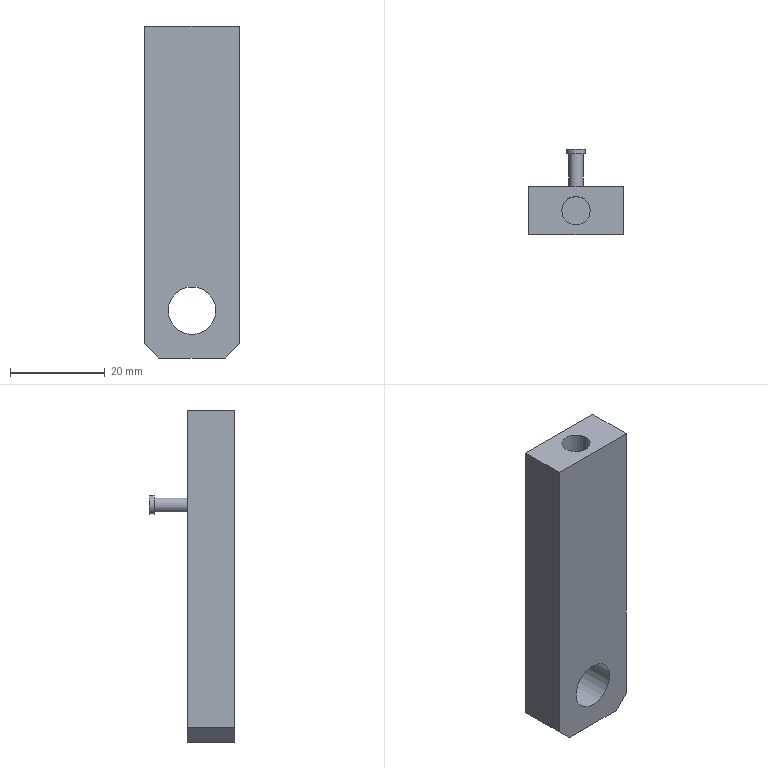Part | NX | features DATUM_CSYS 4, EXTRUDE 3, SKETCH 3, HOLE PACKAGE 1, SIMPLE HOLE 1 | 1 solid | 15 faces | box 20 x 18 x 70 mm | volume 11773 mm3 | plane 11 | cylinder 4 | commonest cylinder face diameters 3 x1 4 x1 6 x1 10 x1
STEP:
#1=CARTESIAN_POINT('',(-10.,5.,0.));
#2=VERTEX_POINT('',#1);
#3=CARTESIAN_POINT('',(-10.,5.,-67.));
#4=VERTEX_POINT('',#3);
#5=CARTESIAN_POINT('',(-10.,5.,0.));
#6=DIRECTION('',(0.,0.,-1.));
#7=VECTOR('',#6,1000.);
#8=LINE('',#5,#7);
#9=EDGE_CURVE('',#2,#4,#8,.T.);
#10=ORIENTED_EDGE('',*,*,#9,.T.);
#11=CARTESIAN_POINT('',(-10.,-5.,-67.));
#12=VERTEX_POINT('',#11);
#13=CARTESIAN_POINT('',(-10.,-5.,-67.));
#14=DIRECTION('',(0.,1.,0.));
#15=VECTOR('',#14,1000.);
#16=LINE('',#13,#15);
#17=EDGE_CURVE('',#12,#4,#16,.T.);
#18=ORIENTED_EDGE('',*,*,#17,.F.);
#19=CARTESIAN_POINT('',(-10.,-5.,0.));
#20=VERTEX_POINT('',#19);
#21=CARTESIAN_POINT('',(-10.,-5.,0.));
#22=DIRECTION('',(0.,0.,-1.));
#23=VECTOR('',#22,1000.);
#24=LINE('',#21,#23);
#25=EDGE_CURVE('',#20,#12,#24,.T.);
#26=ORIENTED_EDGE('',*,*,#25,.F.);
#27=CARTESIAN_POINT('',(-10.,-5.,0.));
#28=DIRECTION('',(0.,1.,0.));
#29=VECTOR('',#28,1000.);
#30=LINE('',#27,#29);
#31=EDGE_CURVE('',#20,#2,#30,.T.);
#32=ORIENTED_EDGE('',*,*,#31,.T.);
#33=EDGE_LOOP('',(#10,#18,#26,#32));
#34=FACE_BOUND('',#33,.T.);
#35=CARTESIAN_POINT('',(-10.,-5.,0.));
#36=DIRECTION('',(1.,0.,0.));
#37=DIRECTION('',(0.,0.,-1.));
#38=AXIS2_PLACEMENT_3D('',#35,#36,#37);
#39=PLANE('',#38);
#40=ADVANCED_FACE('',(#34),#39,.F.);
#41=CARTESIAN_POINT('',(-7.,5.,-70.));
#42=VERTEX_POINT('',#41);
#43=CARTESIAN_POINT('',(-10.,5.,-67.));
#44=DIRECTION('',(0.7071,0.,-0.7071));
#45=VECTOR('',#44,1000.);
#46=LINE('',#43,#45);
#47=EDGE_CURVE('',#4,#42,#46,.T.);
#48=ORIENTED_EDGE('',*,*,#47,.T.);
#49=CARTESIAN_POINT('',(-7.,-5.,-70.));
#50=VERTEX_POINT('',#49);
#51=CARTESIAN_POINT('',(-7.,-5.,-70.));
#52=DIRECTION('',(0.,1.,0.));
#53=VECTOR('',#52,1000.);
#54=LINE('',#51,#53);
#55=EDGE_CURVE('',#50,#42,#54,.T.);
#56=ORIENTED_EDGE('',*,*,#55,.F.);
#57=CARTESIAN_POINT('',(-10.,-5.,-67.));
#58=DIRECTION('',(0.7071,0.,-0.7071));
#59=VECTOR('',#58,1000.);
#60=LINE('',#57,#59);
#61=EDGE_CURVE('',#12,#50,#60,.T.);
#62=ORIENTED_EDGE('',*,*,#61,.F.);
#63=ORIENTED_EDGE('',*,*,#17,.T.);
#64=EDGE_LOOP('',(#48,#56,#62,#63));
#65=FACE_BOUND('',#64,.T.);
#66=CARTESIAN_POINT('',(-10.,-5.,-67.));
#67=DIRECTION('',(0.7071,0.,0.7071));
#68=DIRECTION('',(0.7071,0.,-0.7071));
#69=AXIS2_PLACEMENT_3D('',#66,#67,#68);
#70=PLANE('',#69);
#71=ADVANCED_FACE('',(#65),#70,.F.);
#72=CARTESIAN_POINT('',(7.,5.,-70.));
#73=VERTEX_POINT('',#72);
#74=CARTESIAN_POINT('',(-7.,5.,-70.));
#75=DIRECTION('',(1.,0.,0.));
#76=VECTOR('',#75,1000.);
#77=LINE('',#74,#76);
#78=EDGE_CURVE('',#42,#73,#77,.T.);
#79=ORIENTED_EDGE('',*,*,#78,.T.);
#80=CARTESIAN_POINT('',(7.,-5.,-70.));
#81=VERTEX_POINT('',#80);
#82=CARTESIAN_POINT('',(7.,-5.,-70.));
#83=DIRECTION('',(0.,1.,0.));
#84=VECTOR('',#83,1000.);
#85=LINE('',#82,#84);
#86=EDGE_CURVE('',#81,#73,#85,.T.);
#87=ORIENTED_EDGE('',*,*,#86,.F.);
#88=CARTESIAN_POINT('',(-7.,-5.,-70.));
#89=DIRECTION('',(1.,0.,0.));
#90=VECTOR('',#89,1000.);
#91=LINE('',#88,#90);
#92=EDGE_CURVE('',#50,#81,#91,.T.);
#93=ORIENTED_EDGE('',*,*,#92,.F.);
#94=ORIENTED_EDGE('',*,*,#55,.T.);
#95=EDGE_LOOP('',(#79,#87,#93,#94));
#96=FACE_BOUND('',#95,.T.);
#97=CARTESIAN_POINT('',(-7.,-5.,-70.));
#98=DIRECTION('',(0.,0.,1.));
#99=DIRECTION('',(1.,0.,0.));
#100=AXIS2_PLACEMENT_3D('',#97,#98,#99);
#101=PLANE('',#100);
#102=ADVANCED_FACE('',(#96),#101,.F.);
#103=CARTESIAN_POINT('',(10.,5.,-67.));
#104=VERTEX_POINT('',#103);
#105=CARTESIAN_POINT('',(7.,5.,-70.));
#106=DIRECTION('',(0.7071,0.,0.7071));
#107=VECTOR('',#106,1000.);
#108=LINE('',#105,#107);
#109=EDGE_CURVE('',#73,#104,#108,.T.);
#110=ORIENTED_EDGE('',*,*,#109,.T.);
#111=CARTESIAN_POINT('',(10.,-5.,-67.));
#112=VERTEX_POINT('',#111);
#113=CARTESIAN_POINT('',(10.,-5.,-67.));
#114=DIRECTION('',(0.,1.,0.));
#115=VECTOR('',#114,1000.);
#116=LINE('',#113,#115);
#117=EDGE_CURVE('',#112,#104,#116,.T.);
#118=ORIENTED_EDGE('',*,*,#117,.F.);
#119=CARTESIAN_POINT('',(7.,-5.,-70.));
#120=DIRECTION('',(0.7071,0.,0.7071));
#121=VECTOR('',#120,1000.);
#122=LINE('',#119,#121);
#123=EDGE_CURVE('',#81,#112,#122,.T.);
#124=ORIENTED_EDGE('',*,*,#123,.F.);
#125=ORIENTED_EDGE('',*,*,#86,.T.);
#126=EDGE_LOOP('',(#110,#118,#124,#125));
#127=FACE_BOUND('',#126,.T.);
#128=CARTESIAN_POINT('',(7.,-5.,-70.));
#129=DIRECTION('',(-0.7071,0.,0.7071));
#130=DIRECTION('',(0.7071,0.,0.7071));
#131=AXIS2_PLACEMENT_3D('',#128,#129,#130);
#132=PLANE('',#131);
#133=ADVANCED_FACE('',(#127),#132,.F.);
#134=CARTESIAN_POINT('',(10.,5.,0.));
#135=VERTEX_POINT('',#134);
#136=CARTESIAN_POINT('',(10.,5.,-67.));
#137=DIRECTION('',(0.,0.,1.));
#138=VECTOR('',#137,1000.);
#139=LINE('',#136,#138);
#140=EDGE_CURVE('',#104,#135,#139,.T.);
#141=ORIENTED_EDGE('',*,*,#140,.T.);
#142=CARTESIAN_POINT('',(10.,-5.,0.));
#143=VERTEX_POINT('',#142);
#144=CARTESIAN_POINT('',(10.,-5.,0.));
#145=DIRECTION('',(0.,1.,0.));
#146=VECTOR('',#145,1000.);
#147=LINE('',#144,#146);
#148=EDGE_CURVE('',#143,#135,#147,.T.);
#149=ORIENTED_EDGE('',*,*,#148,.F.);
#150=CARTESIAN_POINT('',(10.,-5.,-67.));
#151=DIRECTION('',(0.,0.,1.));
#152=VECTOR('',#151,1000.);
#153=LINE('',#150,#152);
#154=EDGE_CURVE('',#112,#143,#153,.T.);
#155=ORIENTED_EDGE('',*,*,#154,.F.);
#156=ORIENTED_EDGE('',*,*,#117,.T.);
#157=EDGE_LOOP('',(#141,#149,#155,#156));
#158=FACE_BOUND('',#157,.T.);
#159=CARTESIAN_POINT('',(10.,-5.,-67.));
#160=DIRECTION('',(-1.,0.,0.));
#161=DIRECTION('',(0.,0.,1.));
#162=AXIS2_PLACEMENT_3D('',#159,#160,#161);
#163=PLANE('',#162);
#164=ADVANCED_FACE('',(#158),#163,.F.);
#165=CARTESIAN_POINT('',(-3.,0.,0.));
#166=VERTEX_POINT('',#165);
#167=CARTESIAN_POINT('',(0.,0.,0.));
#168=DIRECTION('',(0.,0.,-1.));
#169=DIRECTION('',(-1.,0.,0.));
#170=AXIS2_PLACEMENT_3D('',#167,#168,#169);
#171=CIRCLE('',#170,3.);
#172=EDGE_CURVE('',#166,#166,#171,.T.);
#173=ORIENTED_EDGE('',*,*,#172,.T.);
#174=EDGE_LOOP('',(#173));
#175=FACE_BOUND('',#174,.T.);
#176=CARTESIAN_POINT('',(10.,5.,0.));
#177=DIRECTION('',(-1.,0.,0.));
#178=VECTOR('',#177,1000.);
#179=LINE('',#176,#178);
#180=EDGE_CURVE('',#135,#2,#179,.T.);
#181=ORIENTED_EDGE('',*,*,#180,.T.);
#182=ORIENTED_EDGE('',*,*,#31,.F.);
#183=CARTESIAN_POINT('',(10.,-5.,0.));
#184=DIRECTION('',(-1.,0.,0.));
#185=VECTOR('',#184,1000.);
#186=LINE('',#183,#185);
#187=EDGE_CURVE('',#143,#20,#186,.T.);
#188=ORIENTED_EDGE('',*,*,#187,.F.);
#189=ORIENTED_EDGE('',*,*,#148,.T.);
#190=EDGE_LOOP('',(#181,#182,#188,#189));
#191=FACE_BOUND('',#190,.T.);
#192=CARTESIAN_POINT('',(10.,-5.,0.));
#193=DIRECTION('',(0.,0.,-1.));
#194=DIRECTION('',(-1.,0.,0.));
#195=AXIS2_PLACEMENT_3D('',#192,#193,#194);
#196=PLANE('',#195);
#197=ADVANCED_FACE('',(#175,#191),#196,.F.);
#198=CARTESIAN_POINT('',(5.,-5.,-60.));
#199=VERTEX_POINT('',#198);
#200=CARTESIAN_POINT('',(0.,-5.,-60.));
#201=DIRECTION('',(0.,-1.,0.));
#202=DIRECTION('',(1.,0.,0.));
#203=AXIS2_PLACEMENT_3D('',#200,#201,#202);
#204=CIRCLE('',#203,5.);
#205=EDGE_CURVE('',#199,#199,#204,.T.);
#206=ORIENTED_EDGE('',*,*,#205,.T.);
#207=EDGE_LOOP('',(#206));
#208=FACE_BOUND('',#207,.T.);
#209=CARTESIAN_POINT('',(5.,5.,-60.));
#210=VERTEX_POINT('',#209);
#211=CARTESIAN_POINT('',(0.,5.,-60.));
#212=DIRECTION('',(0.,-1.,0.));
#213=DIRECTION('',(1.,0.,0.));
#214=AXIS2_PLACEMENT_3D('',#211,#212,#213);
#215=CIRCLE('',#214,5.);
#216=EDGE_CURVE('',#210,#210,#215,.T.);
#217=ORIENTED_EDGE('',*,*,#216,.F.);
#218=EDGE_LOOP('',(#217));
#219=FACE_BOUND('',#218,.T.);
#220=CARTESIAN_POINT('',(0.,-5.,-60.));
#221=DIRECTION('',(0.,1.,0.));
#222=DIRECTION('',(0.,0.,1.));
#223=AXIS2_PLACEMENT_3D('',#220,#221,#222);
#224=CYLINDRICAL_SURFACE('',#223,5.);
#225=ADVANCED_FACE('',(#208,#219),#224,.F.);
#226=ORIENTED_EDGE('',*,*,#25,.T.);
#227=ORIENTED_EDGE('',*,*,#61,.T.);
#228=ORIENTED_EDGE('',*,*,#92,.T.);
#229=ORIENTED_EDGE('',*,*,#123,.T.);
#230=ORIENTED_EDGE('',*,*,#154,.T.);
#231=ORIENTED_EDGE('',*,*,#187,.T.);
#232=EDGE_LOOP('',(#226,#227,#228,#229,#230,#231));
#233=FACE_BOUND('',#232,.T.);
#234=ORIENTED_EDGE('',*,*,#205,.F.);
#235=EDGE_LOOP('',(#234));
#236=FACE_BOUND('',#235,.T.);
#237=CARTESIAN_POINT('',(0.,-5.,-60.));
#238=DIRECTION('',(0.,-1.,0.));
#239=DIRECTION('',(0.,0.,-1.));
#240=AXIS2_PLACEMENT_3D('',#237,#238,#239);
#241=PLANE('',#240);
#242=ADVANCED_FACE('',(#233,#236),#241,.T.);
#243=CARTESIAN_POINT('',(1.5,5.,-20.));
#244=VERTEX_POINT('',#243);
#245=CARTESIAN_POINT('',(0.,5.,-20.));
#246=DIRECTION('',(0.,-1.,0.));
#247=DIRECTION('',(1.,0.,0.));
#248=AXIS2_PLACEMENT_3D('',#245,#246,#247);
#249=CIRCLE('',#248,1.5);
#250=EDGE_CURVE('',#244,#244,#249,.T.);
#251=ORIENTED_EDGE('',*,*,#250,.T.);
#252=EDGE_LOOP('',(#251));
#253=FACE_BOUND('',#252,.T.);
#254=ORIENTED_EDGE('',*,*,#9,.F.);
#255=ORIENTED_EDGE('',*,*,#180,.F.);
#256=ORIENTED_EDGE('',*,*,#140,.F.);
#257=ORIENTED_EDGE('',*,*,#109,.F.);
#258=ORIENTED_EDGE('',*,*,#78,.F.);
#259=ORIENTED_EDGE('',*,*,#47,.F.);
#260=EDGE_LOOP('',(#254,#255,#256,#257,#258,#259));
#261=FACE_BOUND('',#260,.T.);
#262=ORIENTED_EDGE('',*,*,#216,.T.);
#263=EDGE_LOOP('',(#262));
#264=FACE_BOUND('',#263,.T.);
#265=CARTESIAN_POINT('',(0.,5.,-60.));
#266=DIRECTION('',(0.,-1.,0.));
#267=DIRECTION('',(0.,0.,-1.));
#268=AXIS2_PLACEMENT_3D('',#265,#266,#267);
#269=PLANE('',#268);
#270=ADVANCED_FACE('',(#253,#261,#264),#269,.F.);
#271=CARTESIAN_POINT('',(1.5,12.,-20.));
#272=VERTEX_POINT('',#271);
#273=CARTESIAN_POINT('',(0.,12.,-20.));
#274=DIRECTION('',(0.,-1.,0.));
#275=DIRECTION('',(1.,0.,0.));
#276=AXIS2_PLACEMENT_3D('',#273,#274,#275);
#277=CIRCLE('',#276,1.5);
#278=EDGE_CURVE('',#272,#272,#277,.T.);
#279=ORIENTED_EDGE('',*,*,#278,.T.);
#280=EDGE_LOOP('',(#279));
#281=FACE_BOUND('',#280,.T.);
#282=ORIENTED_EDGE('',*,*,#250,.F.);
#283=EDGE_LOOP('',(#282));
#284=FACE_BOUND('',#283,.T.);
#285=CARTESIAN_POINT('',(0.,12.,-20.));
#286=DIRECTION('',(0.,-1.,0.));
#287=DIRECTION('',(0.,0.,-1.));
#288=AXIS2_PLACEMENT_3D('',#285,#286,#287);
#289=CYLINDRICAL_SURFACE('',#288,1.5);
#290=ADVANCED_FACE('',(#281,#284),#289,.T.);
#291=CARTESIAN_POINT('',(-2.,13.,-20.));
#292=VERTEX_POINT('',#291);
#293=CARTESIAN_POINT('',(0.,13.,-20.));
#294=DIRECTION('',(0.,-1.,0.));
#295=DIRECTION('',(-1.,0.,0.));
#296=AXIS2_PLACEMENT_3D('',#293,#294,#295);
#297=CIRCLE('',#296,2.);
#298=EDGE_CURVE('',#292,#292,#297,.T.);
#299=ORIENTED_EDGE('',*,*,#298,.T.);
#300=EDGE_LOOP('',(#299));
#301=FACE_BOUND('',#300,.T.);
#302=CARTESIAN_POINT('',(-2.,12.,-20.));
#303=VERTEX_POINT('',#302);
#304=CARTESIAN_POINT('',(0.,12.,-20.));
#305=DIRECTION('',(0.,-1.,0.));
#306=DIRECTION('',(-1.,0.,0.));
#307=AXIS2_PLACEMENT_3D('',#304,#305,#306);
#308=CIRCLE('',#307,2.);
#309=EDGE_CURVE('',#303,#303,#308,.T.);
#310=ORIENTED_EDGE('',*,*,#309,.F.);
#311=EDGE_LOOP('',(#310));
#312=FACE_BOUND('',#311,.T.);
#313=CARTESIAN_POINT('',(0.,13.,-20.));
#314=DIRECTION('',(0.,-1.,0.));
#315=DIRECTION('',(0.,0.,-1.));
#316=AXIS2_PLACEMENT_3D('',#313,#314,#315);
#317=CYLINDRICAL_SURFACE('',#316,2.);
#318=ADVANCED_FACE('',(#301,#312),#317,.T.);
#319=ORIENTED_EDGE('',*,*,#298,.F.);
#320=EDGE_LOOP('',(#319));
#321=FACE_BOUND('',#320,.T.);
#322=CARTESIAN_POINT('',(0.,13.,-20.));
#323=DIRECTION('',(0.,-1.,0.));
#324=DIRECTION('',(0.,0.,-1.));
#325=AXIS2_PLACEMENT_3D('',#322,#323,#324);
#326=PLANE('',#325);
#327=ADVANCED_FACE('',(#321),#326,.F.);
#328=ORIENTED_EDGE('',*,*,#278,.F.);
#329=EDGE_LOOP('',(#328));
#330=FACE_BOUND('',#329,.T.);
#331=ORIENTED_EDGE('',*,*,#309,.T.);
#332=EDGE_LOOP('',(#331));
#333=FACE_BOUND('',#332,.T.);
#334=CARTESIAN_POINT('',(0.,12.,-20.));
#335=DIRECTION('',(0.,-1.,0.));
#336=DIRECTION('',(0.,0.,-1.));
#337=AXIS2_PLACEMENT_3D('',#334,#335,#336);
#338=PLANE('',#337);
#339=ADVANCED_FACE('',(#330,#333),#338,.T.);
#340=CARTESIAN_POINT('',(-3.,0.,-50.));
#341=VERTEX_POINT('',#340);
#342=CARTESIAN_POINT('',(0.,0.,-50.));
#343=DIRECTION('',(0.,0.,-1.));
#344=DIRECTION('',(-1.,0.,0.));
#345=AXIS2_PLACEMENT_3D('',#342,#343,#344);
#346=CIRCLE('',#345,3.);
#347=EDGE_CURVE('',#341,#341,#346,.F.);
#348=ORIENTED_EDGE('',*,*,#347,.T.);
#349=EDGE_LOOP('',(#348));
#350=FACE_BOUND('',#349,.T.);
#351=CARTESIAN_POINT('',(0.,0.,-50.));
#352=DIRECTION('',(0.,0.,-1.));
#353=DIRECTION('',(-1.,0.,0.));
#354=AXIS2_PLACEMENT_3D('',#351,#352,#353);
#355=PLANE('',#354);
#356=ADVANCED_FACE('',(#350),#355,.F.);
#357=ORIENTED_EDGE('',*,*,#347,.F.);
#358=EDGE_LOOP('',(#357));
#359=FACE_BOUND('',#358,.T.);
#360=ORIENTED_EDGE('',*,*,#172,.F.);
#361=EDGE_LOOP('',(#360));
#362=FACE_BOUND('',#361,.T.);
#363=CARTESIAN_POINT('',(0.,0.,0.));
#364=DIRECTION('',(0.,0.,-1.));
#365=DIRECTION('',(-1.,0.,0.));
#366=AXIS2_PLACEMENT_3D('',#363,#364,#365);
#367=CYLINDRICAL_SURFACE('',#366,3.);
#368=ADVANCED_FACE('',(#359,#362),#367,.F.);
#369=CLOSED_SHELL('',(#40,#71,#102,#133,#164,#197,#225,#242,#270,#290,#318,#327,#339,#356,#368));
#370=MANIFOLD_SOLID_BREP('',#369);
#371=(LENGTH_UNIT()NAMED_UNIT(*)SI_UNIT(.MILLI.,.METRE.));
#372=UNCERTAINTY_MEASURE_WITH_UNIT(LENGTH_MEASURE(0.00001),#371,'','');
#373=(NAMED_UNIT(*)PLANE_ANGLE_UNIT()SI_UNIT($,.RADIAN.));
#374=(NAMED_UNIT(*)SI_UNIT($,.STERADIAN.)SOLID_ANGLE_UNIT());
#375=(GEOMETRIC_REPRESENTATION_CONTEXT(3)GLOBAL_UNCERTAINTY_ASSIGNED_CONTEXT((#372))GLOBAL_UNIT_ASSIGNED_CONTEXT((#371,#373,#374))REPRESENTATION_CONTEXT('',''));
#376=ADVANCED_BREP_SHAPE_REPRESENTATION('',(#370),#375);